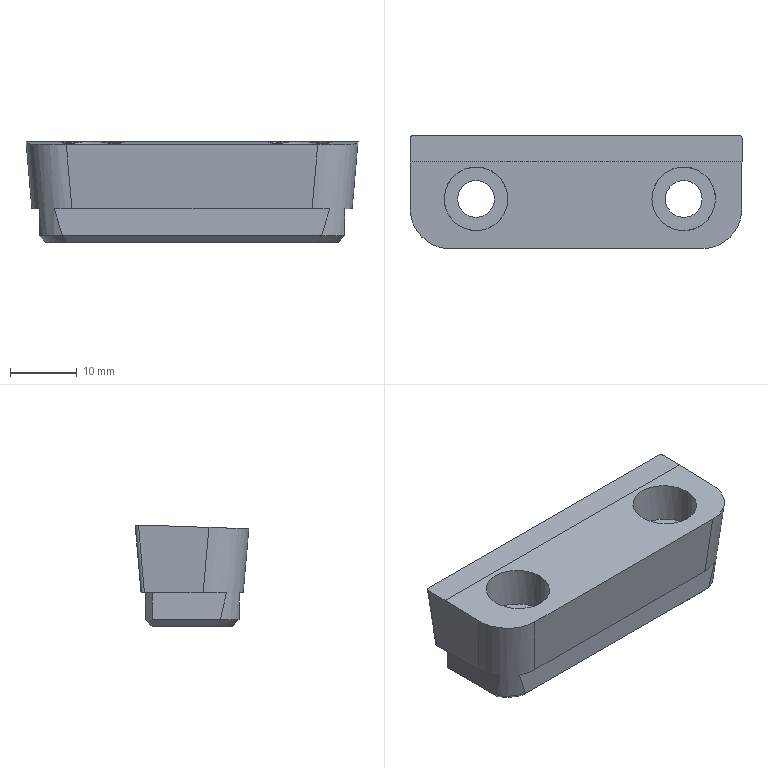Part | Creo | 1 solid | 45 faces | box 49.562 x 16.961 x 15 mm | volume 9228 mm3 | plane 23 | cylinder 16 | cone 4 | spline 2 | commonest cylinder face diameters 5.5 x4 8 x4 9.5 x4 1 x2 12 x2